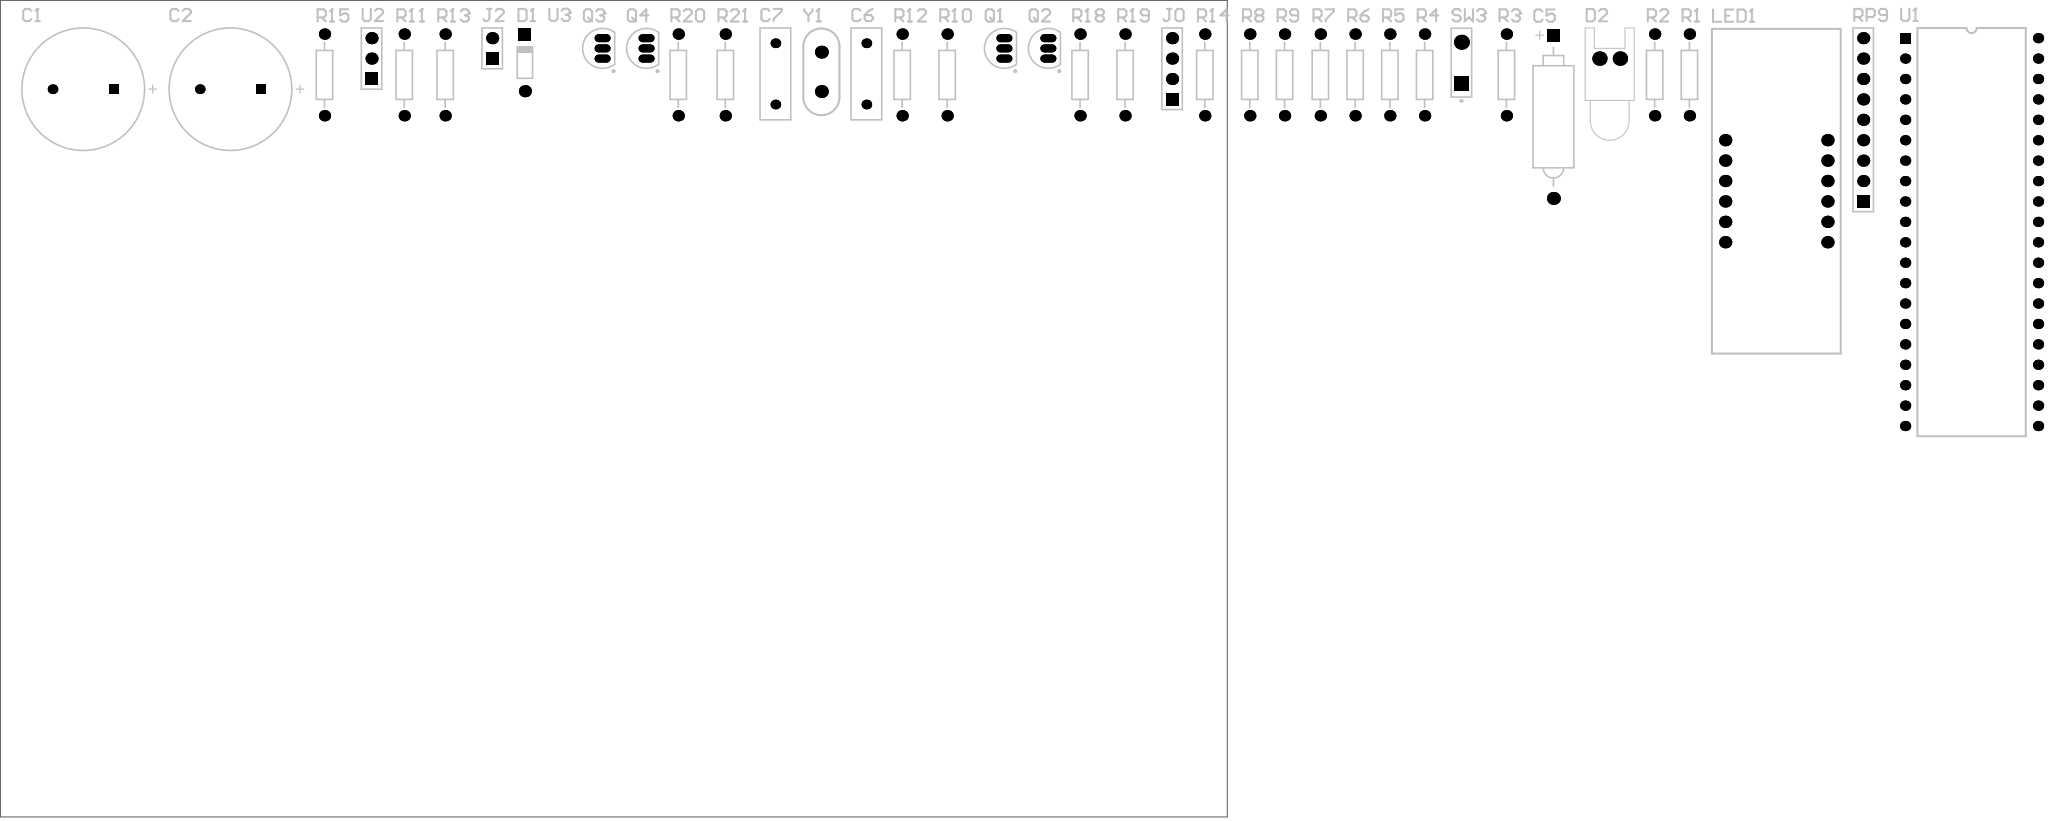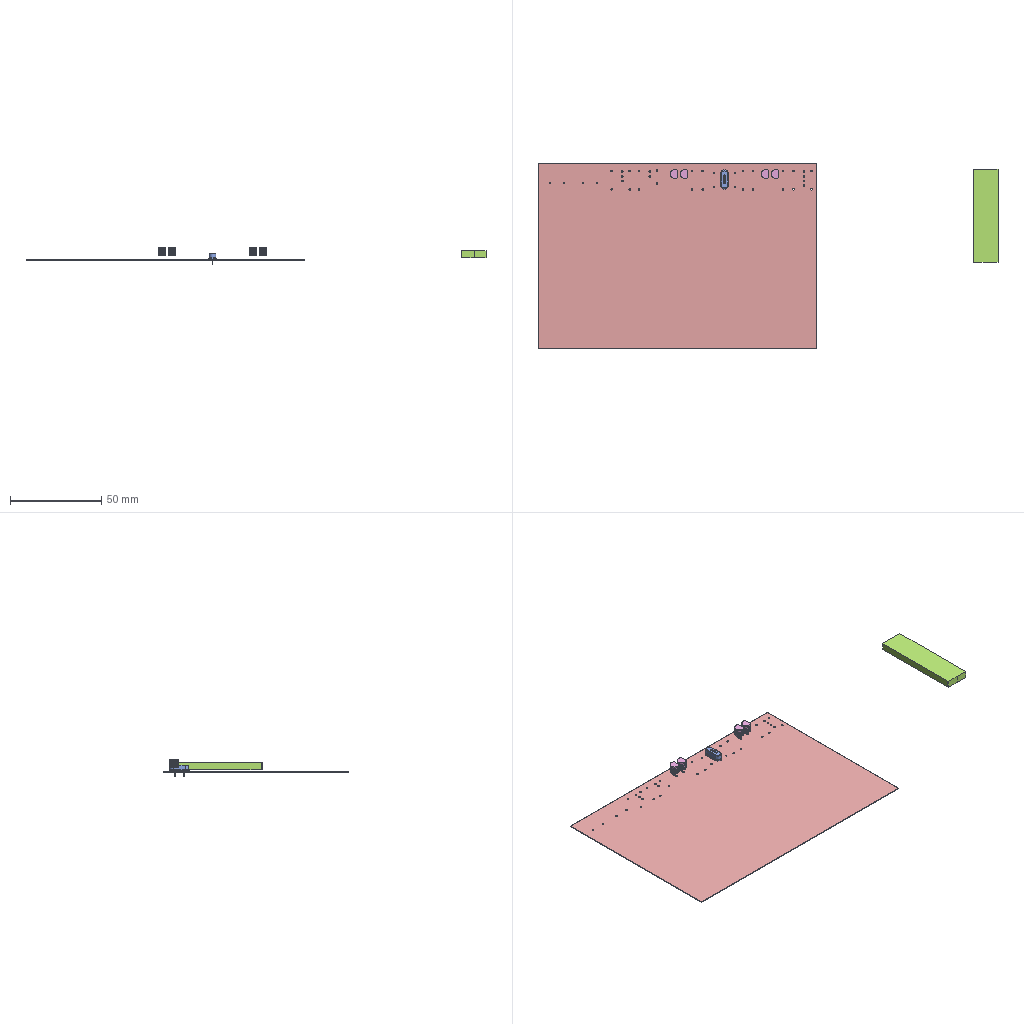Circuit board layout | Altium Designer | box 251.6 x 101.6 x 9.8 mm
Part placement:
Designator,Comment,Layer,Footprint,Center-X(mm),Center-Y(mm),Rotation
Y1,Component_1,TopLayer,LC-HC-49S,127.381,118.11,90
U3,7805,TopLayer,PCBComponent_1,0,0,90
U2,AH49E,TopLayer,HDR1X3,71.501,119.761,90
U1,89c51,TopLayer,89c51,270.256,98.171,0
SW3,SW-PB,TopLayer,SPST-2,206.883,119.253,90
RP9,20k,TopLayer,HDR1X9,256.794,112.141,90
R21,Res2,TopLayer,AXIAL-0.4,115.443,117.729,90
R20,Res2,TopLayer,AXIAL-0.4,109.601,117.729,90
R19,Res2,TopLayer,AXIAL-0.4,165.1,117.729,90
R18,Res2,TopLayer,AXIAL-0.4,159.512,117.729,90
R15,Res2,TopLayer,AXIAL-0.4,65.659,117.729,90
R14,Res2,TopLayer,AXIAL-0.4,175.006,117.729,90
R13,Res2,TopLayer,AXIAL-0.4,80.645,117.729,90
R12,Res2,TopLayer,AXIAL-0.4,137.414,117.729,90
R11,Res2,TopLayer,AXIAL-0.4,75.565,117.729,90
R10,Res2,TopLayer,AXIAL-0.4,143.002,117.729,90
R9,Res2,TopLayer,AXIAL-0.4,184.912,117.729,90
R8,Res2,TopLayer,AXIAL-0.4,180.594,117.729,90
R7,Res2,TopLayer,AXIAL-0.4,189.357,117.729,90
R6,Res2,TopLayer,AXIAL-0.4,193.675,117.729,90
R5,Res2,TopLayer,AXIAL-0.4,197.993,117.729,90
R4,Res2,TopLayer,AXIAL-0.4,202.311,117.729,90
R3,Res2,TopLayer,AXIAL-0.4,212.471,117.729,90
R2,Res2,TopLayer,AXIAL-0.4,230.886,117.729,90
R1,Res2,TopLayer,AXIAL-0.4,235.204,117.729,90
Q4,2N3906,TopLayer,TO-92A,105.664,121.031,0
Q3,2N3906,TopLayer,TO-92A,100.203,121.031,0
Q2,2N3906,TopLayer,TO-92A,155.575,121.031,0
Q1,2N3906,TopLayer,TO-92A,150.114,121.031,0
LED1,Dpy Red-CA,TopLayer,四位数码管,246,103.258,90
J2,Header 2,TopLayer,HDR1X2,86.487,121.031,90
J0,Header 4,TopLayer,HDR1X4,170.942,118.491,90
D2,LED0,TopLayer,LED-0,225.298,119.761,0
D1,Diode 1N914,TopLayer,DO-35,90.551,119.253,90
C7,Cap,TopLayer,RAD-0.3,121.666,117.856,90
C6,Cap,TopLayer,RAD-0.3,132.969,117.856,90
C5,Cap Pol2,TopLayer,POLAR0.8,218.313,112.522,90
C2,Cap Pol1,TopLayer,RB7.6-15,53.975,115.951,0
C1,Cap Pol1,TopLayer,RB7.6-15,35.687,115.951,0